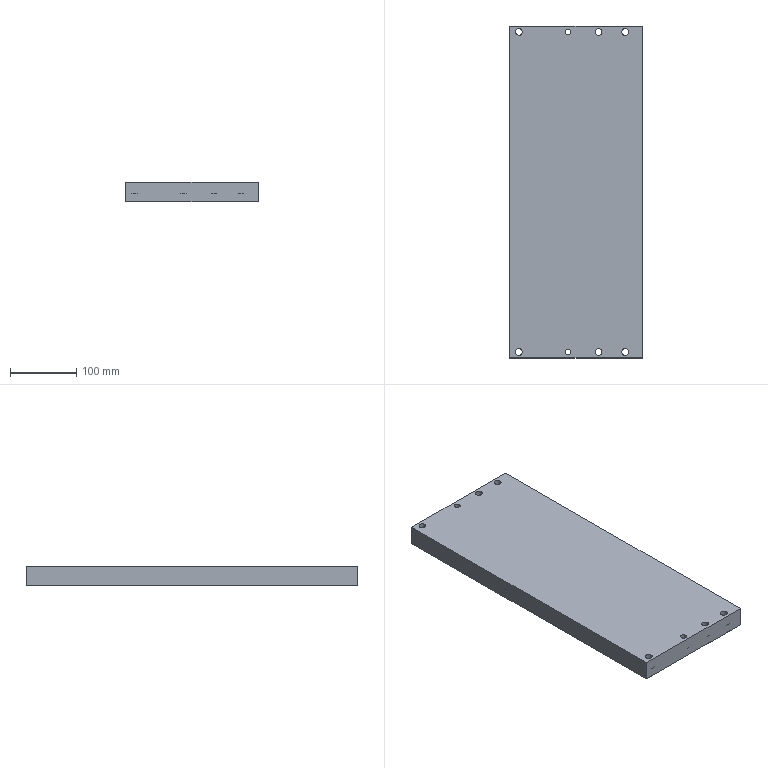NC program | NX | posted with a generic post | part box 200 x 500 x 30 mm
Whole program:
N10 G17 G21 G94 G90
(DRILLING , TOOL : ZXZ)
N12 T01 M6
N14 G54
N16 G17 G0 G90 X-60.811 Y60.811 S1000 M3
N18 G43 Z50. H1
N20 G94 G81 G99 Z-21.5 F60. R-18.5
N22 G0 Z30.
N24 G81 X60.811 Z-21.5 R-18.5
N26 G0 Z30.
N28 G81 Y-60.811 Z-21.5 R-18.5
N30 G0 Z30.
N32 G81 X-60.811 Z-21.5 R-18.5
N34 G0 Z30.
N36 G80
N38 G0 X-60.811 Y-60.811 Z50.
N40 M5
(DRILLING_COPY , TOOL : D10.5Z)
N42 T02 M6
N44 G54
N46 G17 G0 G90 X-60.811 Y60.811 S650 M3
N48 G43 Z50. H2
N50 G94 G83 G99 Z-50. F60. Q3. R-18.5
N52 G0 Z30.
N54 G83 X60.811 Z-50. Q3. R-18.5
N56 G0 Z30.
N58 G83 Y-60.811 Z-50. Q3. R-18.5
N60 G0 Z30.
N62 G83 X-60.811 Z-50. Q3. R-18.5
N64 G0 Z30.
N66 G80
N68 G0 X-60.811 Y-60.811 Z50.
N70 M5
(DRILLING_COPY_COPY , TOOL : D18R0)
N72 T03 M6
N74 G54
N76 G17 G0 G90 X-60.811 Y60.811 S400 M3
N78 G43 Z50. H3
N80 G94 G83 G99 Z-32. F30. Q1.5 R-18.5
N82 G0 Z30.
N84 G83 X60.811 Z-32. Q1.5 R-18.5
N86 G0 Z30.
N88 G83 Y-60.811 Z-32. Q1.5 R-18.5
N90 G0 Z30.
N92 G83 X-60.811 Z-32. Q1.5 R-18.5
N94 G0 Z30.
N96 G80
N98 G0 X-60.811 Y-60.811 Z50.
N100 M5
(PLANAR_MILL , TOOL : D10R0)
N102 T05 M6
N104 G54
N106 G17 G0 G90 X-110.76 Y26.674 S2500 M3
N108 G43 Z80. H5
N110 G94 G1 Z-19.95 F3000.
N112 G41 X-109.775 Y26.5 F400. D5
N114 X-102.775
N116 X102.775
N118 X109.775
N120 G40
N122 X110.76 Y26.674
N124 G0 Z80.
N126 Y-26.674
N128 G1 Z-19.95 F3000.
N130 G41 X109.775 Y-26.5 F400.
N132 X102.775
N134 X-102.775
N136 X-109.775
N138 G40
N140 X-110.76 Y-26.674
N142 G0 Z80.
N144 M5
(PLANAR_MILL_COPY , TOOL : DJ-6)
N146 T06 M6
N148 G54
N150 G17 G0 G90 X-60.811 Y60.811 S3000 M3
N152 G43 Z60. H6
N154 G94 G1 Z-22. F3000.
N156 G41 X-53.811 F800. D6
N158 G3 X-60.811 Y67.811 R7.
N160 X-53.811 Y60.811 R-7.
N162 G40
N164 G1 X-60.811
N166 G0 Z60.
N168 Y-60.811
N170 G1 Z-22. F3000.
N172 G41 X-53.811 F800.
N174 G3 X-60.811 Y-53.811 R7.
N176 X-53.811 Y-60.811 R-7.
N178 G40
N180 G1 X-60.811
N182 G0 Z60.
N184 X60.811
N186 G1 Z-22. F3000.
N188 G41 X67.811 F800.
N190 G3 X60.811 Y-53.811 R7.
N192 X67.811 Y-60.811 R-7.
N194 G40
N196 G1 X60.811
N198 G0 Z60.
N200 Y60.811
N202 G1 Z-22. F3000.
N204 G41 X67.811 F800.
N206 G3 X60.811 Y67.811 R7.
N208 X67.811 Y60.811 R-7.
N210 G40
N212 G1 X60.811
N214 G0 Z60.
(PLANAR_MILL_COPY_COPY , TOOL : DJ-6)
N216 Z80.
N218 X111.76 Y-23.674
N220 G1 Z-2. F3000.
N222 G41 X110.775 Y-23.5 F800.
N224 X102.775
N226 X-102.775
N228 X-110.775
N230 G40
N232 X-111.76 Y-23.674
N234 G0 Z80.
N236 Y23.674
N238 G1 Z-2. F3000.
N240 G41 X-110.775 Y23.5 F800.
N242 X-102.775
N244 X102.775
N246 X110.775
N248 G40
N250 X111.76 Y23.674
N252 G0 Z80.
N254 M5
(DRILLING_COPY_1 , TOOL : ZXZ)
N256 T01 M6
N258 G54
N260 G17 G0 G90 X71.98 Y-10. S1000 M3
N262 G43 Z80. H1
N264 G94 G81 G99 Z-1.5 F60. R1.5
N266 G0 Z80.
N268 G81 X41.98 Z-1.5 R1.5
N270 G0 Z80.
N272 G81 X11.98 Z-1.5 R1.5
N274 G0 Z80.
N276 G80
N278 G0 X11.98 Y-10. Z80.
N280 M5
(DRILLING_COPY_1_COPY , TOOL : D8.5Z)
N282 T02 M6
N284 G54
N286 G17 G0 G90 X71.98 Y-10. S800 M3
N288 G43 Z80. H2
N290 G94 G83 G99 Z-21.5 F60. Q4.25 R1.5
N292 G0 Z80.
N294 G83 X41.98 Z-21.5 Q4.25 R1.5
N296 G0 Z80.
N298 G83 X11.98 Z-21.5 Q4.25 R1.5
N300 G0 Z80.
N302 G80
N304 G0 X11.98 Y-10. Z80.
N306 M5
(DRILLING_COPY_1_COPY_1 , TOOL : ZXZ)
N308 T01 M6
N310 G54
N312 G17 G0 G90 X86. Y-10. S1000 M3
N314 G43 Z80. H1
N316 G94 G81 G99 Z-1.5 F60. R1.5
N318 G0 Z80.
N320 G81 X72. Z-1.5 R1.5
N322 G0 Z80.
N324 G81 X42. Z-1.5 R1.5
N326 G0 Z80.
N328 G81 X12. Z-1.5 R1.5
N330 G0 Z80.
N332 G81 X-34. Z-1.5 R1.5
N334 G0 Z80.
N336 G81 X-74. Z-1.5 R1.5
N338 G0 Z80.
N340 G80
N342 G0 X-74. Y-10. Z80.
N344 M5
(DRILLING_COPY_1_COPY_COPY_1 , TOOL : D8.5Z)
N346 T02 M6
N348 G54
N350 G17 G0 G90 X72. Y-10. S800 M3
N352 G43 Z80. H2
N354 G94 G83 G99 Z-25. F60. Q4.25 R1.5
N356 G0 Z80.
N358 G83 X42. Z-25. Q4.25 R1.5
N360 G0 Z80.
N362 G83 X12. Z-25. Q4.25 R1.5
N364 G0 Z80.
N366 G80
N368 G0 X12. Y-10. Z80.
N370 M5
(DRILLING_COPY_1_COPY_COPY_COPY , TOOL : D10.3Z)
N372 T04 M6
N374 G54
N376 G17 G0 G90 X86. Y-10. S500 M3
N378 G43 Z80. H4
N380 G94 G83 G99 Z-21.5 F22. Q3. R1.5
N382 G0 Z80.
N384 G83 X-34. Z-21.5 Q3. R1.5
N386 G0 Z80.
N388 G83 X-74. Z-21.5 Q3. R1.5
N390 G0 Z80.
N392 G80
N394 G0 X-74. Y-10. Z80.
N396 M5
(DJ , TOOL : DJ-12)
N398 T01 M6
N400 G54
N402 G17 G0 G90 X-241. Y86. S2000 M3
N404 G43 Z30. H1
N406 G94 G81 G99 Z-4. F120. R3.
N408 G0 Z30.
N410 G81 Y12. Z-4. R3.
N412 G0 Z30.
N414 G81 Y-34. Z-4. R3.
N416 G0 Z30.
N418 G81 Y-74. Z-4. R3.
N420 G0 Z30.
N422 G81 X241. Z-4. R3.
N424 G0 Z30.
N426 G81 Y-34. Z-4. R3.
N428 G0 Z30.
N430 G81 Y12. Z-4. R3.
N432 G0 Z30.
N434 G81 Y86. Z-4. R3.
N436 G0 Z30.
N438 G80
N440 G0 X241. Y86. Z30.
N442 M5
(11ZT , TOOL : D11Z)
N444 T02 M6
N446 G54
N448 G17 G0 G90 X-241. Y86. S2000 M3
N450 G43 Z30. H2
N452 G94 G83 G99 Z-34. F120. Q5.5 R3.
N454 G0 Z30.
N456 G83 Y12. Z-34. Q5.5 R3.
N458 G0 Z30.
N460 G83 Y-34. Z-34. Q5.5 R3.
N462 G0 Z30.
N464 G83 Y-74. Z-34. Q5.5 R3.
N466 G0 Z30.
N468 G83 X241. Z-34. Q5.5 R3.
N470 G0 Z30.
N472 G83 Y-34. Z-34. Q5.5 R3.
N474 G0 Z30.
N476 G83 Y12. Z-34. Q5.5 R3.
N478 G0 Z30.
N480 G83 Y86. Z-34. Q5.5 R3.
N482 G0 Z30.
N484 G80
N486 G0 X241. Y86. Z30.
N488 M5
(PLANAR_MILL_1 , TOOL : D10)
N490 T03 M6
N492 G54
N494 G17 G0 G90 X243.997 Y-75.605 S3500 M3
N496 G43 Z30. H3
N498 Z0.3
N500 G94 G3 X243.997 Y-75.605 Z-0.446 I-2.997 J1.605 F300.
N502 X243.997 Y-75.605 Z-1.192 I-2.997 J1.605
N504 X243.997 Y-75.605 Z-1.938 I-2.997 J1.605
N506 X243.997 Y-75.605 Z-2.684 I-2.997 J1.605
N508 X243.997 Y-75.605 Z-3.43 I-2.997 J1.605
N510 X243.997 Y-75.605 Z-4.176 I-2.997 J1.605
N512 X243.997 Y-75.605 Z-4.922 I-2.997 J1.605
N514 X243.997 Y-75.605 Z-5.668 I-2.997 J1.605
N516 X243.997 Y-75.605 Z-6.414 I-2.997 J1.605
N518 X243.997 Y-75.605 Z-7.16 I-2.997 J1.605
N520 X243.997 Y-75.605 Z-7.906 I-2.997 J1.605
N522 X243.997 Y-75.605 Z-8.652 I-2.997 J1.605
N524 X243.997 Y-75.605 Z-9.398 I-2.997 J1.605
N526 X243.997 Y-75.605 Z-10.144 I-2.997 J1.605
N528 X243.997 Y-75.605 Z-10.89 I-2.997 J1.605
N530 X243.997 Y-75.605 Z-11.636 I-2.997 J1.605
N532 X243.997 Y-75.605 Z-12.382 I-2.997 J1.605
N534 X241. Y-77.4 Z-13. R-3.4
N536 X244.4 Y-74. R3.4
N538 X241. Y-77.4 R-3.4
N540 G0 Z30.
N542 X243.997 Y-35.605
N544 Z0.3
N546 G3 X243.997 Y-35.605 Z-0.446 I-2.997 J1.605
N548 X243.997 Y-35.605 Z-1.192 I-2.997 J1.605
N550 X243.997 Y-35.605 Z-1.938 I-2.997 J1.605
N552 X243.997 Y-35.605 Z-2.684 I-2.997 J1.605
N554 X243.997 Y-35.605 Z-3.43 I-2.997 J1.605
N556 X243.997 Y-35.605 Z-4.176 I-2.997 J1.605
N558 X243.997 Y-35.605 Z-4.922 I-2.997 J1.605
N560 X243.997 Y-35.605 Z-5.668 I-2.997 J1.605
N562 X243.997 Y-35.605 Z-6.414 I-2.997 J1.605
N564 X243.997 Y-35.605 Z-7.16 I-2.997 J1.605
N566 X243.997 Y-35.605 Z-7.906 I-2.997 J1.605
N568 X243.997 Y-35.605 Z-8.652 I-2.997 J1.605
N570 X243.997 Y-35.605 Z-9.398 I-2.997 J1.605
N572 X243.997 Y-35.605 Z-10.144 I-2.997 J1.605
N574 X243.997 Y-35.605 Z-10.89 I-2.997 J1.605
N576 X243.997 Y-35.605 Z-11.636 I-2.997 J1.605
N578 X243.997 Y-35.605 Z-12.382 I-2.997 J1.605
N580 X241. Y-37.4 Z-13. R-3.4
N582 X244.4 Y-34. R3.4
N584 X241. Y-37.4 R-3.4
N586 G0 Z30.
N588 X243.997 Y10.395
N590 Z0.3
N592 G3 X243.997 Y10.395 Z-0.446 I-2.997 J1.605
N594 X243.997 Y10.395 Z-1.192 I-2.997 J1.605
N596 X243.997 Y10.395 Z-1.938 I-2.997 J1.605
N598 X243.997 Y10.395 Z-2.684 I-2.997 J1.605
N600 X243.997 Y10.395 Z-3.43 I-2.997 J1.605
N602 X243.997 Y10.395 Z-4.176 I-2.997 J1.605
N604 X243.997 Y10.395 Z-4.922 I-2.997 J1.605
N606 X243.997 Y10.395 Z-5.668 I-2.997 J1.605
N608 X243.997 Y10.395 Z-6.414 I-2.997 J1.605
N610 X243.997 Y10.395 Z-7.16 I-2.997 J1.605
N612 X243.997 Y10.395 Z-7.906 I-2.997 J1.605
N614 X243.997 Y10.395 Z-8.652 I-2.997 J1.605
N616 X243.997 Y10.395 Z-9.398 I-2.997 J1.605
N618 X243.997 Y10.395 Z-10.144 I-2.997 J1.605
N620 X243.997 Y10.395 Z-10.89 I-2.997 J1.605
N622 X243.997 Y10.395 Z-11.636 I-2.997 J1.605
N624 X243.997 Y10.395 Z-12.382 I-2.997 J1.605
N626 X241. Y8.6 Z-13. R-3.4
N628 X244.4 Y12. R3.4
N630 X241. Y8.6 R-3.4
N632 G0 Z30.
N634 X238.003 Y87.605
N636 Z0.3
N638 G3 X238.003 Y87.605 Z-0.446 I2.997 J-1.605
N640 X238.003 Y87.605 Z-1.192 I2.997 J-1.605
N642 X238.003 Y87.605 Z-1.938 I2.997 J-1.605
N644 X238.003 Y87.605 Z-2.684 I2.997 J-1.605
N646 X238.003 Y87.605 Z-3.43 I2.997 J-1.605
N648 X238.003 Y87.605 Z-4.176 I2.997 J-1.605
N650 X238.003 Y87.605 Z-4.922 I2.997 J-1.605
N652 X238.003 Y87.605 Z-5.668 I2.997 J-1.605
N654 X238.003 Y87.605 Z-6.414 I2.997 J-1.605
N656 X238.003 Y87.605 Z-7.16 I2.997 J-1.605
N658 X238.003 Y87.605 Z-7.906 I2.997 J-1.605
N660 X238.003 Y87.605 Z-8.652 I2.997 J-1.605
N662 X238.003 Y87.605 Z-9.398 I2.997 J-1.605
N664 X238.003 Y87.605 Z-10.144 I2.997 J-1.605
N666 X238.003 Y87.605 Z-10.89 I2.997 J-1.605
N668 X238.003 Y87.605 Z-11.636 I2.997 J-1.605
N670 X238.003 Y87.605 Z-12.382 I2.997 J-1.605
N672 X241. Y89.4 Z-13. R-3.4
N674 X237.6 Y86. R3.4
N676 X241. Y89.4 R-3.4
N678 G0 Z30.
N680 X-243.997 Y87.605
N682 Z0.3
N684 G3 X-243.997 Y87.605 Z-0.446 I2.997 J-1.605
N686 X-243.997 Y87.605 Z-1.192 I2.997 J-1.605
N688 X-243.997 Y87.605 Z-1.938 I2.997 J-1.605
N690 X-243.997 Y87.605 Z-2.684 I2.997 J-1.605
N692 X-243.997 Y87.605 Z-3.43 I2.997 J-1.605
N694 X-243.997 Y87.605 Z-4.176 I2.997 J-1.605
N696 X-243.997 Y87.605 Z-4.922 I2.997 J-1.605
N698 X-243.997 Y87.605 Z-5.668 I2.997 J-1.605
N700 X-243.997 Y87.605 Z-6.414 I2.997 J-1.605
N702 X-243.997 Y87.605 Z-7.16 I2.997 J-1.605
N704 X-243.997 Y87.605 Z-7.906 I2.997 J-1.605
N706 X-243.997 Y87.605 Z-8.652 I2.997 J-1.605
N708 X-243.997 Y87.605 Z-9.398 I2.997 J-1.605
N710 X-243.997 Y87.605 Z-10.144 I2.997 J-1.605
N712 X-243.997 Y87.605 Z-10.89 I2.997 J-1.605
N714 X-243.997 Y87.605 Z-11.636 I2.997 J-1.605
N716 X-243.997 Y87.605 Z-12.382 I2.997 J-1.605
N718 X-241. Y89.4 Z-13. R-3.4
N720 X-244.4 Y86. R3.4
N722 X-241. Y89.4 R-3.4
N724 G0 Z30.
N726 X-238.003 Y10.395
N728 Z0.3
N730 G3 X-238.003 Y10.395 Z-0.446 I-2.997 J1.605
N732 X-238.003 Y10.395 Z-1.192 I-2.997 J1.605
N734 X-238.003 Y10.395 Z-1.938 I-2.997 J1.605
N736 X-238.003 Y10.395 Z-2.684 I-2.997 J1.605
N738 X-238.003 Y10.395 Z-3.43 I-2.997 J1.605
N740 X-238.003 Y10.395 Z-4.176 I-2.997 J1.605
N742 X-238.003 Y10.395 Z-4.922 I-2.997 J1.605
N744 X-238.003 Y10.395 Z-5.668 I-2.997 J1.605
N746 X-238.003 Y10.395 Z-6.414 I-2.997 J1.605
N748 X-238.003 Y10.395 Z-7.16 I-2.997 J1.605
N750 X-238.003 Y10.395 Z-7.906 I-2.997 J1.605
N752 X-238.003 Y10.395 Z-8.652 I-2.997 J1.605
N754 X-238.003 Y10.395 Z-9.398 I-2.997 J1.605
N756 X-238.003 Y10.395 Z-10.144 I-2.997 J1.605
N758 X-238.003 Y10.395 Z-10.89 I-2.997 J1.605
N760 X-238.003 Y10.395 Z-11.636 I-2.997 J1.605
N762 X-238.003 Y10.395 Z-12.382 I-2.997 J1.605
N764 X-241. Y8.6 Z-13. R-3.4
N766 X-237.6 Y12. R3.4
N768 X-241. Y8.6 R-3.4
N770 G0 Z30.
N772 X-238.003 Y-35.605
N774 Z0.3
N776 G3 X-238.003 Y-35.605 Z-0.446 I-2.997 J1.605
N778 X-238.003 Y-35.605 Z-1.192 I-2.997 J1.605
N780 X-238.003 Y-35.605 Z-1.938 I-2.997 J1.605
N782 X-238.003 Y-35.605 Z-2.684 I-2.997 J1.605
N784 X-238.003 Y-35.605 Z-3.43 I-2.997 J1.605
N786 X-238.003 Y-35.605 Z-4.176 I-2.997 J1.605
N788 X-238.003 Y-35.605 Z-4.922 I-2.997 J1.605
N790 X-238.003 Y-35.605 Z-5.668 I-2.997 J1.605
N792 X-238.003 Y-35.605 Z-6.414 I-2.997 J1.605
N794 X-238.003 Y-35.605 Z-7.16 I-2.997 J1.605
N796 X-238.003 Y-35.605 Z-7.906 I-2.997 J1.605
N798 X-238.003 Y-35.605 Z-8.652 I-2.997 J1.605
N800 X-238.003 Y-35.605 Z-9.398 I-2.997 J1.605
N802 X-238.003 Y-35.605 Z-10.144 I-2.997 J1.605
N804 X-238.003 Y-35.605 Z-10.89 I-2.997 J1.605
N806 X-238.003 Y-35.605 Z-11.636 I-2.997 J1.605
N808 X-238.003 Y-35.605 Z-12.382 I-2.997 J1.605
N810 X-241. Y-37.4 Z-13. R-3.4
N812 X-237.6 Y-34. R3.4
N814 X-241. Y-37.4 R-3.4
N816 G0 Z30.
N818 X-238.003 Y-75.605
N820 Z0.3
N822 G3 X-238.003 Y-75.605 Z-0.446 I-2.997 J1.605
N824 X-238.003 Y-75.605 Z-1.192 I-2.997 J1.605
N826 X-238.003 Y-75.605 Z-1.938 I-2.997 J1.605
N828 X-238.003 Y-75.605 Z-2.684 I-2.997 J1.605
N830 X-238.003 Y-75.605 Z-3.43 I-2.997 J1.605
N832 X-238.003 Y-75.605 Z-4.176 I-2.997 J1.605
N834 X-238.003 Y-75.605 Z-4.922 I-2.997 J1.605
N836 X-238.003 Y-75.605 Z-5.668 I-2.997 J1.605
N838 X-238.003 Y-75.605 Z-6.414 I-2.997 J1.605
N840 X-238.003 Y-75.605 Z-7.16 I-2.997 J1.605
N842 X-238.003 Y-75.605 Z-7.906 I-2.997 J1.605
N844 X-238.003 Y-75.605 Z-8.652 I-2.997 J1.605
N846 X-238.003 Y-75.605 Z-9.398 I-2.997 J1.605
N848 X-238.003 Y-75.605 Z-10.144 I-2.997 J1.605
N850 X-238.003 Y-75.605 Z-10.89 I-2.997 J1.605
N852 X-238.003 Y-75.605 Z-11.636 I-2.997 J1.605
N854 X-238.003 Y-75.605 Z-12.382 I-2.997 J1.605
N856 X-241. Y-77.4 Z-13. R-3.4
N858 X-237.6 Y-74. R3.4
N860 X-241. Y-77.4 R-3.4
N862 G0 Z30.
(PLANAR_MILL_1_COPY , TOOL : D10)
N864 X-239. Y87.5
N866 Z-10.
N868 G1 Z-13.
N870 G3 X-241. Y89.5 R2.
N872 X-244.5 Y86. R3.5
N874 X-241. Y89.5 R-3.5
N876 X-243. Y87.5 R2.
N878 G1 Z-10.
N880 G0 Z30.
N882 Y10.5
N884 Z-10.
N886 G1 Z-13.
N888 G3 X-241. Y8.5 R2.
N890 X-237.5 Y12. R3.5
N892 X-241. Y8.5 R-3.5
N894 X-239. Y10.5 R2.
N896 G1 Z-10.
N898 G0 Z30.
N900 X-243. Y-35.5
N902 Z-10.
N904 G1 Z-13.
N906 G3 X-241. Y-37.5 R2.
N908 X-237.5 Y-34. R3.5
N910 X-241. Y-37.5 R-3.5
N912 X-239. Y-35.5 R2.
N914 G1 Z-10.
N916 G0 Z30.
N918 X-243. Y-75.5
N920 Z-10.
N922 G1 Z-13.
N924 G3 X-241. Y-77.5 R2.
N926 X-237.5 Y-74. R3.5
N928 X-241. Y-77.5 R-3.5
N930 X-239. Y-75.5 R2.
N932 G1 Z-10.
N934 G0 Z30.
N936 X239.
N938 Z-10.
N940 G1 Z-13.
N942 G3 X241. Y-77.5 R2.
N944 X244.5 Y-74. R3.5
N946 X241. Y-77.5 R-3.5
N948 X243. Y-75.5 R2.
N950 G1 Z-10.
N952 G0 Z30.
N954 X239. Y-35.5
N956 Z-10.
N958 G1 Z-13.
N960 G3 X241. Y-37.5 R2.
N962 X244.5 Y-34. R3.5
N964 X241. Y-37.5 R-3.5
N966 X243. Y-35.5 R2.
N968 G1 Z-10.
N970 G0 Z30.
N972 X239. Y10.5
N974 Z-10.
N976 G1 Z-13.
N978 G3 X241. Y8.5 R2.
N980 X244.5 Y12. R3.5
N982 X241. Y8.5 R-3.5
N984 X243. Y10.5 R2.
N986 G1 Z-10.
N988 G0 Z30.
N990 Y87.5
N992 Z-10.
N994 G1 Z-13.
N996 G3 X241. Y89.5 R2.
N998 X237.5 Y86. R3.5
N1000 X241. Y89.5 R-3.5
N1002 X239. Y87.5 R2.
N1004 G1 Z-10.
N1006 G0 Z30.
N1008 M5
(DJ-J , TOOL : DJ-6)
N1010 T01 M6
N1012 G54
N1014 G17 G0 G90 X-244. Y-76.795 S3000 M3
N1016 G43 Z30. H1
N1018 Z1.5
N1020 G94 G1 Z-1.5 F1000.
N1022 Y-78.1
N1024 G3 X-241. Y-81.1 R3.
N1026 X-233.9 Y-74. R7.1
N1028 X-241. Y-81.1 R-7.1
N1030 X-238. Y-78.1 R3.
N1032 G1 Y-76.795
N1034 Z1.5
N1036 G0 Z30.
N1038 X-244. Y-36.795
N1040 Z1.5
N1042 G1 Z-1.5
N1044 Y-38.1
N1046 G3 X-241. Y-41.1 R3.
N1048 X-233.9 Y-34. R7.1
N1050 X-241. Y-41.1 R-7.1
N1052 X-238. Y-38.1 R3.
N1054 G1 Y-36.795
N1056 Z1.5
N1058 G0 Z30.
N1060 X-244. Y9.205
N1062 Z1.5
N1064 G1 Z-1.5
N1066 Y7.9
N1068 G3 X-241. Y4.9 R3.
N1070 X-233.9 Y12. R7.1
N1072 X-241. Y4.9 R-7.1
N1074 X-238. Y7.9 R3.
N1076 G1 Y9.205
N1078 Z1.5
N1080 G0 Z30.
N1082 Y88.795
N1084 Z1.5
N1086 G1 Z-1.5
N1088 Y90.1
N1090 G3 X-241. Y93.1 R3.
N1092 X-248.1 Y86. R7.1
N1094 X-241. Y93.1 R-7.1
N1096 X-244. Y90.1 R3.
N1098 G1 Y88.795
N1100 Z1.5
N1102 G0 Z30.
N1104 X244.
N1106 Z1.5
N1108 G1 Z-1.5
N1110 Y90.1
N1112 G3 X241. Y93.1 R3.
N1114 X233.9 Y86. R7.1
N1116 X241. Y93.1 R-7.1
N1118 X238. Y90.1 R3.
N1120 G1 Y88.795
N1122 Z1.5
N1124 G0 Z30.
N1126 Y9.205
N1128 Z1.5
N1130 G1 Z-1.5
N1132 Y7.9
N1134 G3 X241. Y4.9 R3.
N1136 X248.1 Y12. R7.1
N1138 X241. Y4.9 R-7.1
N1140 X244. Y7.9 R3.
N1142 G1 Y9.205
N1144 Z1.5
N1146 G0 Z30.
N1148 X238. Y-36.795
N1150 Z1.5
N1152 G1 Z-1.5
N1154 Y-38.1
N1156 G3 X241. Y-41.1 R3.
N1158 X248.1 Y-34. R7.1
N1160 X241. Y-41.1 R-7.1
N1162 X244. Y-38.1 R3.
N1164 G1 Y-36.795
N1166 Z1.5
N1168 G0 Z30.
N1170 X238. Y-76.795
N1172 Z1.5
N1174 G1 Z-1.5
N1176 Y-78.1
N1178 G3 X241. Y-81.1 R3.
N1180 X248.1 Y-74. R7.1
N1182 X241. Y-81.1 R-7.1
N1184 X244. Y-78.1 R3.
N1186 G1 Y-76.795
N1188 Z1.5
N1190 G0 Z30.
(DJ-J_COPY , TOOL : DJ-6)
N1192 X240.4 Y-77.15
N1194 Z-11.5
N1196 G1 Z-14.5
N1198 G3 X241. Y-77.75 R0.6
N1200 X244.75 Y-74. R3.75
N1202 X241. Y-77.75 R-3.75
N1204 X241.6 Y-77.15 R0.6
N1206 G1 Z-11.5
N1208 G0 Z30.
N1210 X240.4 Y-37.15
N1212 Z-11.5
N1214 G1 Z-14.5
N1216 G3 X241. Y-37.75 R0.6
N1218 X244.75 Y-34. R3.75
N1220 X241. Y-37.75 R-3.75
N1222 X241.6 Y-37.15 R0.6
N1224 G1 Z-11.5
N1226 G0 Z30.
N1228 X240.4 Y9.7
N1230 Z-11.5
N1232 G1 Z-14.5
N1234 G3 X241. Y9.1 R0.6
N1236 X243.9 Y12. R2.9
N1238 X241. Y9.1 R-2.9
N1240 X241.6 Y9.7 R0.6
N1242 G1 Z-11.5
N1244 G0 Z30.
N1246 X240.4 Y82.85
N1248 Z-11.5
N1250 G1 Z-14.5
N1252 G3 X241. Y82.25 R0.6
N1254 X244.75 Y86. R3.75
N1256 X241. Y82.25 R-3.75
N1258 X241.6 Y82.85 R0.6
N1260 G1 Z-11.5
N1262 G0 Z30.
N1264 X-241.6
N1266 Z-11.5
N1268 G1 Z-14.5
N1270 G3 X-241. Y82.25 R0.6
N1272 X-237.25 Y86. R3.75
N1274 X-241. Y82.25 R-3.75
N1276 X-240.4 Y82.85 R0.6
N1278 G1 Z-11.5
N1280 G0 Z30.
N1282 X-241.6 Y9.7
N1284 Z-11.5
N1286 G1 Z-14.5
N1288 G3 X-241. Y9.1 R0.6
N1290 X-238.1 Y12. R2.9
N1292 X-241. Y9.1 R-2.9
N1294 X-240.4 Y9.7 R0.6
N1296 G1 Z-11.5
N1298 G0 Z30.
N1300 X-241.6 Y-37.15
N1302 Z-11.5
N1304 G1 Z-14.5
N1306 G3 X-241. Y-37.75 R0.6
N1308 X-237.25 Y-34. R3.75
N1310 X-241. Y-37.75 R-3.75
N1312 X-240.4 Y-37.15 R0.6
N1314 G1 Z-11.5
N1316 G0 Z30.
N1318 X-241.6 Y-77.15
N1320 Z-11.5
N1322 G1 Z-14.5
N1324 G3 X-241. Y-77.75 R0.6
N1326 X-237.25 Y-74. R3.75
N1328 X-241. Y-77.75 R-3.75
N1330 X-240.4 Y-77.15 R0.6
N1332 G1 Z-11.5
N1334 G0 Z30.
N1336 M5
N1338 M2